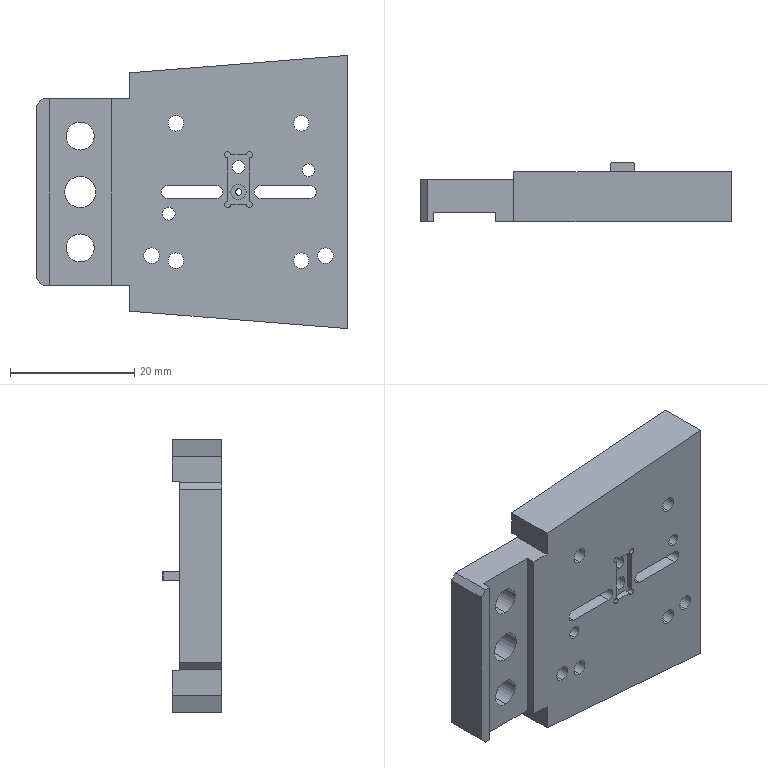Part | SolidWorks | features HoleWzd 10, ICE 8, Chamfer 2, Cut 1, Extrusion 1 | 1 solid | 137 faces | box 50 x 9.6 x 44 mm | volume 11717 mm3 | cylinder 70 | plane 39 | cone 28 | commonest cylinder face diameters 2.05 x14 2.5 x14 1.2 x12 1 x8 1.6 x8 2 x4